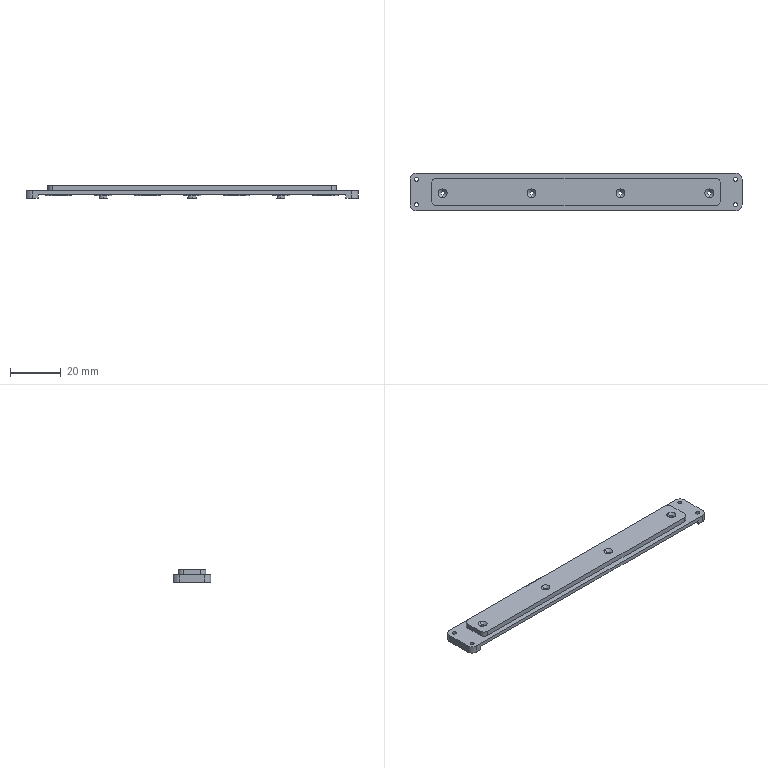Part | 1 solid | 160 faces | box 130.666 x 14.95 x 5 mm | volume 5506 mm3 | cylinder 74 | plane 64 | cone 22 | commonest cylinder face diameters 5 x20 2 x16 1.6 x14 1.5 x8 3.2 x6 7 x6